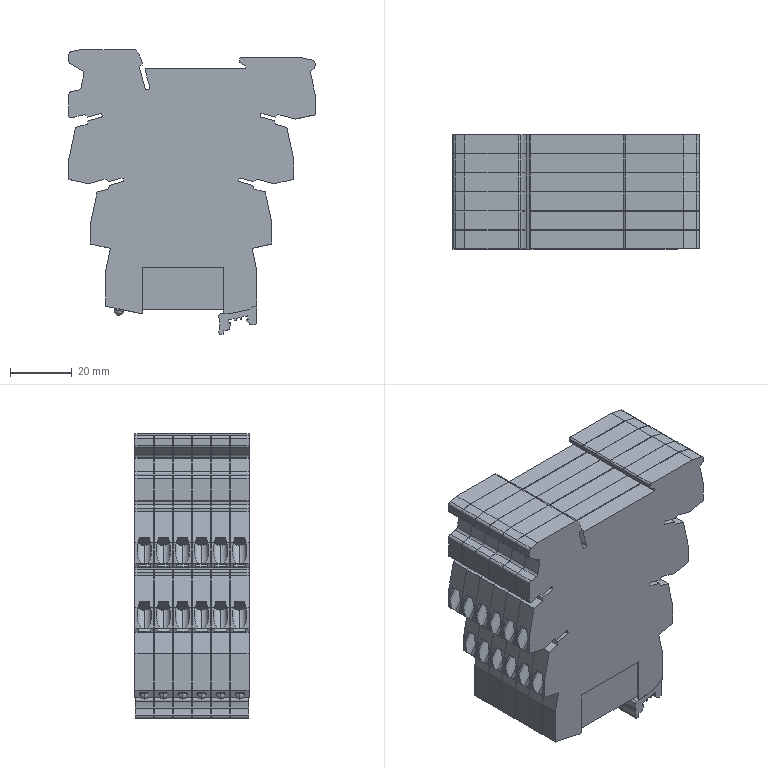Part | SolidWorks | features BaseBody 1 | 1 solid | 1468 faces | box 80 x 37.1 x 92.55 mm | volume 180588 mm3 | plane 1038 | cylinder 406 | cone 12 | sphere 12 | commonest cylinder face diameters 4.8 x120 0.6 x114 2 x54 1 x46 1.6 x30 0.34 x18